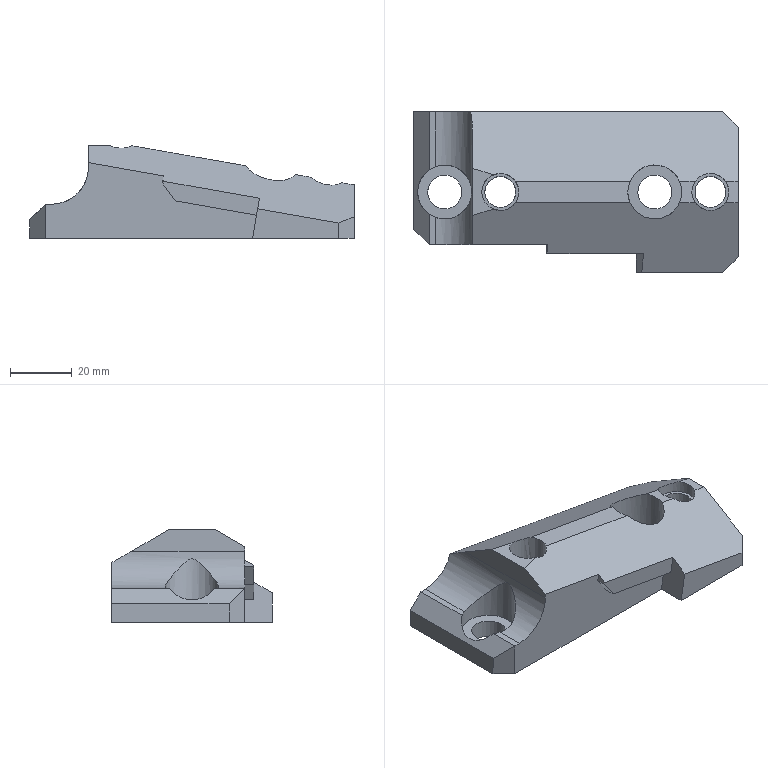Part | NX | features solid 2 | 1 solid | 37 faces | box 105 x 52 x 30.034 mm | volume 76466 mm3 | plane 28 | cylinder 7 | spline 2 | commonest cylinder face diameters 10 x2 11 x2 17.5 x2 24 x1
STEP:
#1=CARTESIAN_POINT('',(216.,165.542,-18.966));
#2=VERTEX_POINT('',#1);
#3=CARTESIAN_POINT('',(216.,129.,-18.966));
#4=VERTEX_POINT('',#3);
#5=CARTESIAN_POINT('',(216.,172.,-18.966));
#6=DIRECTION('',(0.,-1.,0.));
#7=VECTOR('',#6,1000.);
#8=LINE('',#5,#7);
#9=EDGE_CURVE('',#2,#4,#8,.T.);
#10=ORIENTED_EDGE('',*,*,#9,.F.);
#11=CARTESIAN_POINT('',(215.421,172.,-22.65));
#12=VERTEX_POINT('',#11);
#13=CARTESIAN_POINT('',(204.,169.152,-18.966));
#14=DIRECTION('',(0.1504,0.5,0.8529));
#15=DIRECTION('',(0.08682,-0.866,0.4924));
#16=AXIS2_PLACEMENT_3D('',#13,#14,#15);
#17=ELLIPSE('',#16,24.,12.);
#18=EDGE_CURVE('',#12,#2,#17,.F.);
#19=ORIENTED_EDGE('',*,*,#18,.F.);
#20=CARTESIAN_POINT('',(204.,172.,-30.966));
#21=VERTEX_POINT('',#20);
#22=CARTESIAN_POINT('',(204.,172.,-18.966));
#23=DIRECTION('',(0.,-1.,0.));
#24=DIRECTION('',(1.,0.,0.));
#25=AXIS2_PLACEMENT_3D('',#22,#23,#24);
#26=CIRCLE('',#25,12.);
#27=EDGE_CURVE('',#21,#12,#26,.T.);
#28=ORIENTED_EDGE('',*,*,#27,.F.);
#29=CARTESIAN_POINT('',(204.,154.22,-30.966));
#30=VERTEX_POINT('',#29);
#31=CARTESIAN_POINT('',(204.,172.,-30.966));
#32=DIRECTION('',(0.,-1.,0.));
#33=VECTOR('',#32,1000.);
#34=LINE('',#31,#33);
#35=EDGE_CURVE('',#21,#30,#34,.T.);
#36=ORIENTED_EDGE('',*,*,#35,.T.);
#37=CARTESIAN_POINT('',(204.,137.78,-30.966));
#38=VERTEX_POINT('',#37);
#39=CARTESIAN_POINT('',(204.,137.78,-30.966));
#40=CARTESIAN_POINT('',(205.575,137.206,-30.966));
#41=CARTESIAN_POINT('',(208.988,137.058,-30.263));
#42=CARTESIAN_POINT('',(212.178,138.742,-27.95));
#43=CARTESIAN_POINT('',(213.938,140.565,-25.79));
#44=CARTESIAN_POINT('',(214.896,142.091,-24.109));
#45=CARTESIAN_POINT('',(215.432,143.518,-22.69));
#46=CARTESIAN_POINT('',(215.694,144.818,-21.684));
#47=CARTESIAN_POINT('',(215.781,146.05,-21.25));
#48=CARTESIAN_POINT('',(215.682,147.258,-21.737));
#49=CARTESIAN_POINT('',(215.413,148.543,-22.746));
#50=CARTESIAN_POINT('',(214.875,149.952,-24.156));
#51=CARTESIAN_POINT('',(213.901,151.482,-25.843));
#52=CARTESIAN_POINT('',(212.158,153.267,-27.963));
#53=CARTESIAN_POINT('',(208.962,154.947,-30.274));
#54=CARTESIAN_POINT('',(205.569,154.792,-30.966));
#55=CARTESIAN_POINT('',(204.,154.22,-30.966));
#56=B_SPLINE_CURVE_WITH_KNOTS('',3,(#39,#40,#41,#42,#43,#44,#45,#46,#47,#48,#49,#50,#51,#52,#53,#54,#55),.UNSPECIFIED.,.F.,.F.,(4,1,1,1,1,1,1,1,1,1,1,1,1,1,4),(0.,0.004955,0.009911,0.01239,0.01487,0.01734,0.01858,0.01982,0.02106,0.0223,0.02478,0.02725,0.02973,0.03469,0.03964),.UNSPECIFIED.);
#57=EDGE_CURVE('',#38,#30,#56,.T.);
#58=ORIENTED_EDGE('',*,*,#57,.F.);
#59=CARTESIAN_POINT('',(204.,129.,-30.966));
#60=VERTEX_POINT('',#59);
#61=CARTESIAN_POINT('',(204.,172.,-30.966));
#62=DIRECTION('',(0.,-1.,0.));
#63=VECTOR('',#62,1000.);
#64=LINE('',#61,#63);
#65=EDGE_CURVE('',#38,#60,#64,.T.);
#66=ORIENTED_EDGE('',*,*,#65,.T.);
#67=CARTESIAN_POINT('',(204.,129.,-18.966));
#68=DIRECTION('',(0.,-1.,0.));
#69=DIRECTION('',(0.,0.,-1.));
#70=AXIS2_PLACEMENT_3D('',#67,#68,#69);
#71=CIRCLE('',#70,12.);
#72=EDGE_CURVE('',#60,#4,#71,.T.);
#73=ORIENTED_EDGE('',*,*,#72,.T.);
#74=EDGE_LOOP('',(#10,#19,#28,#36,#58,#66,#73));
#75=FACE_BOUND('',#74,.T.);
#76=CARTESIAN_POINT('',(204.,172.,-18.966));
#77=DIRECTION('',(0.,-1.,0.));
#78=DIRECTION('',(0.,0.,1.));
#79=AXIS2_PLACEMENT_3D('',#76,#77,#78);
#80=CYLINDRICAL_SURFACE('',#79,12.);
#81=ADVANCED_FACE('',(#75),#80,.F.);
#82=CARTESIAN_POINT('',(244.012,129.,-29.844));
#83=VERTEX_POINT('',#82);
#84=CARTESIAN_POINT('',(270.401,129.,-34.497));
#85=VERTEX_POINT('',#84);
#86=CARTESIAN_POINT('',(194.772,129.,-21.162));
#87=DIRECTION('',(0.9848,0.,-0.1736));
#88=VECTOR('',#87,1000.);
#89=LINE('',#86,#88);
#90=EDGE_CURVE('',#83,#85,#89,.T.);
#91=ORIENTED_EDGE('',*,*,#90,.T.);
#92=CARTESIAN_POINT('',(270.401,126.,-34.497));
#93=VERTEX_POINT('',#92);
#94=CARTESIAN_POINT('',(270.401,120.,-34.497));
#95=DIRECTION('',(0.,1.,0.));
#96=VECTOR('',#95,1000.);
#97=LINE('',#94,#96);
#98=EDGE_CURVE('',#93,#85,#97,.T.);
#99=ORIENTED_EDGE('',*,*,#98,.F.);
#100=CARTESIAN_POINT('',(244.012,126.,-29.844));
#101=VERTEX_POINT('',#100);
#102=CARTESIAN_POINT('',(194.772,126.,-21.162));
#103=DIRECTION('',(0.9848,0.,-0.1736));
#104=VECTOR('',#103,1000.);
#105=LINE('',#102,#104);
#106=EDGE_CURVE('',#101,#93,#105,.T.);
#107=ORIENTED_EDGE('',*,*,#106,.F.);
#108=CARTESIAN_POINT('',(244.012,126.,-29.844));
#109=DIRECTION('',(0.,-1.,0.));
#110=VECTOR('',#109,1000.);
#111=LINE('',#108,#110);
#112=EDGE_CURVE('',#83,#101,#111,.T.);
#113=ORIENTED_EDGE('',*,*,#112,.F.);
#114=EDGE_LOOP('',(#91,#99,#107,#113));
#115=FACE_BOUND('',#114,.T.);
#116=CARTESIAN_POINT('',(194.772,120.,-21.162));
#117=DIRECTION('',(-0.1736,0.,-0.9848));
#118=DIRECTION('',(-0.9848,0.,0.1736));
#119=AXIS2_PLACEMENT_3D('',#116,#117,#118);
#120=PLANE('',#119);
#121=ADVANCED_FACE('',(#115),#120,.T.);
#122=CARTESIAN_POINT('',(269.078,120.,-42.));
#123=VERTEX_POINT('',#122);
#124=CARTESIAN_POINT('',(297.,120.,-42.));
#125=VERTEX_POINT('',#124);
#126=CARTESIAN_POINT('',(166.772,120.,-42.));
#127=DIRECTION('',(1.,0.,0.));
#128=VECTOR('',#127,1000.);
#129=LINE('',#126,#128);
#130=EDGE_CURVE('',#123,#125,#129,.T.);
#131=ORIENTED_EDGE('',*,*,#130,.T.);
#132=CARTESIAN_POINT('',(297.,120.,-37.034));
#133=VERTEX_POINT('',#132);
#134=CARTESIAN_POINT('',(297.,120.,-42.966));
#135=DIRECTION('',(0.,0.,-1.));
#136=VECTOR('',#135,1000.);
#137=LINE('',#134,#136);
#138=EDGE_CURVE('',#133,#125,#137,.T.);
#139=ORIENTED_EDGE('',*,*,#138,.F.);
#140=CARTESIAN_POINT('',(270.769,120.,-32.409));
#141=VERTEX_POINT('',#140);
#142=CARTESIAN_POINT('',(172.845,120.,-15.142));
#143=DIRECTION('',(0.9848,0.,-0.1736));
#144=VECTOR('',#143,1000.);
#145=LINE('',#142,#144);
#146=EDGE_CURVE('',#141,#133,#145,.T.);
#147=ORIENTED_EDGE('',*,*,#146,.F.);
#148=CARTESIAN_POINT('',(259.982,120.,-93.586));
#149=DIRECTION('',(0.1736,0.,0.9848));
#150=VECTOR('',#149,1000.);
#151=LINE('',#148,#150);
#152=EDGE_CURVE('',#123,#141,#151,.T.);
#153=ORIENTED_EDGE('',*,*,#152,.F.);
#154=EDGE_LOOP('',(#131,#139,#147,#153));
#155=FACE_BOUND('',#154,.T.);
#156=CARTESIAN_POINT('',(166.772,120.,-49.585));
#157=DIRECTION('',(0.,-1.,0.));
#158=DIRECTION('',(0.,0.,1.));
#159=AXIS2_PLACEMENT_3D('',#156,#157,#158);
#160=PLANE('',#159);
#161=ADVANCED_FACE('',(#155),#160,.T.);
#162=CARTESIAN_POINT('',(302.,142.536,-24.704));
#163=VERTEX_POINT('',#162);
#164=CARTESIAN_POINT('',(302.,125.,-34.985));
#165=VERTEX_POINT('',#164);
#166=CARTESIAN_POINT('',(302.,130.815,-31.576));
#167=DIRECTION('',(0.,-0.8627,-0.5058));
#168=VECTOR('',#167,1000.);
#169=LINE('',#166,#168);
#170=EDGE_CURVE('',#163,#165,#169,.T.);
#171=ORIENTED_EDGE('',*,*,#170,.F.);
#172=CARTESIAN_POINT('',(297.897,142.536,-23.981));
#173=VERTEX_POINT('',#172);
#174=CARTESIAN_POINT('',(175.104,142.536,-2.329));
#175=DIRECTION('',(0.9848,0.,-0.1736));
#176=VECTOR('',#175,1000.);
#177=LINE('',#174,#176);
#178=EDGE_CURVE('',#173,#163,#177,.T.);
#179=ORIENTED_EDGE('',*,*,#178,.F.);
#180=CARTESIAN_POINT('',(288.103,142.536,-22.254));
#181=VERTEX_POINT('',#180);
#182=CARTESIAN_POINT('',(297.897,142.536,-23.981));
#183=CARTESIAN_POINT('',(297.358,141.77,-24.335));
#184=CARTESIAN_POINT('',(295.85,140.432,-24.853));
#185=CARTESIAN_POINT('',(292.773,139.747,-24.712));
#186=CARTESIAN_POINT('',(289.937,140.598,-23.713));
#187=CARTESIAN_POINT('',(288.601,141.828,-22.757));
#188=CARTESIAN_POINT('',(288.103,142.536,-22.254));
#189=B_SPLINE_CURVE_WITH_KNOTS('',3,(#182,#183,#184,#185,#186,#187,#188),.UNSPECIFIED.,.F.,.F.,(4,1,1,1,4),(0.006466,0.009441,0.01242,0.01539,0.01837),.UNSPECIFIED.);
#190=EDGE_CURVE('',#173,#181,#189,.T.);
#191=ORIENTED_EDGE('',*,*,#190,.T.);
#192=CARTESIAN_POINT('',(283.035,142.536,-21.36));
#193=VERTEX_POINT('',#192);
#194=CARTESIAN_POINT('',(175.104,142.536,-2.329));
#195=DIRECTION('',(0.9848,0.,-0.1736));
#196=VECTOR('',#195,1000.);
#197=LINE('',#194,#196);
#198=EDGE_CURVE('',#193,#181,#197,.T.);
#199=ORIENTED_EDGE('',*,*,#198,.F.);
#200=CARTESIAN_POINT('',(266.965,142.536,-18.527));
#201=VERTEX_POINT('',#200);
#202=CARTESIAN_POINT('',(275.,146.,-17.912));
#203=DIRECTION('',(0.1504,-0.5,0.8529));
#204=DIRECTION('',(0.2456,-0.8167,-0.5221));
#205=AXIS2_PLACEMENT_3D('',#202,#203,#204);
#206=ELLIPSE('',#205,10.259,8.75);
#207=EDGE_CURVE('',#193,#201,#206,.F.);
#208=ORIENTED_EDGE('',*,*,#207,.T.);
#209=CARTESIAN_POINT('',(229.897,142.536,-11.99));
#210=VERTEX_POINT('',#209);
#211=CARTESIAN_POINT('',(175.104,142.536,-2.329));
#212=DIRECTION('',(0.9848,0.,-0.1736));
#213=VECTOR('',#212,1000.);
#214=LINE('',#211,#213);
#215=EDGE_CURVE('',#210,#201,#214,.T.);
#216=ORIENTED_EDGE('',*,*,#215,.F.);
#217=CARTESIAN_POINT('',(222.769,140.434,-11.966));
#218=VERTEX_POINT('',#217);
#219=CARTESIAN_POINT('',(229.897,142.536,-11.99));
#220=CARTESIAN_POINT('',(229.158,141.486,-12.476));
#221=CARTESIAN_POINT('',(226.837,139.774,-13.07));
#222=CARTESIAN_POINT('',(223.955,139.958,-12.454));
#223=CARTESIAN_POINT('',(222.769,140.434,-11.966));
#224=B_SPLINE_CURVE_WITH_KNOTS('',3,(#219,#220,#221,#222,#223),.UNSPECIFIED.,.F.,.F.,(4,1,4),(0.0002423,0.004332,0.008422),.UNSPECIFIED.);
#225=EDGE_CURVE('',#210,#218,#224,.T.);
#226=ORIENTED_EDGE('',*,*,#225,.T.);
#227=CARTESIAN_POINT('',(216.,138.398,-11.966));
#228=VERTEX_POINT('',#227);
#229=CARTESIAN_POINT('',(171.676,125.067,-11.966));
#230=DIRECTION('',(-0.9576,-0.288,0.));
#231=VECTOR('',#230,1000.);
#232=LINE('',#229,#231);
#233=EDGE_CURVE('',#218,#228,#232,.T.);
#234=ORIENTED_EDGE('',*,*,#233,.T.);
#235=CARTESIAN_POINT('',(216.,129.,-17.476));
#236=VERTEX_POINT('',#235);
#237=CARTESIAN_POINT('',(216.,124.198,-20.29));
#238=DIRECTION('',(0.,-0.8627,-0.5058));
#239=VECTOR('',#238,1000.);
#240=LINE('',#237,#239);
#241=EDGE_CURVE('',#228,#236,#240,.T.);
#242=ORIENTED_EDGE('',*,*,#241,.T.);
#243=CARTESIAN_POINT('',(240.359,129.,-21.771));
#244=VERTEX_POINT('',#243);
#245=CARTESIAN_POINT('',(173.747,129.,-10.025));
#246=DIRECTION('',(-0.9848,0.,0.1736));
#247=VECTOR('',#246,1000.);
#248=LINE('',#245,#247);
#249=EDGE_CURVE('',#244,#236,#248,.T.);
#250=ORIENTED_EDGE('',*,*,#249,.F.);
#251=CARTESIAN_POINT('',(240.058,126.,-23.476));
#252=VERTEX_POINT('',#251);
#253=CARTESIAN_POINT('',(239.545,120.885,-26.385));
#254=DIRECTION('',(0.08682,0.866,0.4924));
#255=VECTOR('',#254,1000.);
#256=LINE('',#253,#255);
#257=EDGE_CURVE('',#252,#244,#256,.T.);
#258=ORIENTED_EDGE('',*,*,#257,.F.);
#259=CARTESIAN_POINT('',(271.37,126.,-28.998));
#260=VERTEX_POINT('',#259);
#261=CARTESIAN_POINT('',(173.446,126.,-11.731));
#262=DIRECTION('',(0.9848,0.,-0.1736));
#263=VECTOR('',#262,1000.);
#264=LINE('',#261,#263);
#265=EDGE_CURVE('',#252,#260,#264,.T.);
#266=ORIENTED_EDGE('',*,*,#265,.T.);
#267=CARTESIAN_POINT('',(270.857,120.885,-31.906));
#268=DIRECTION('',(0.08682,0.866,0.4924));
#269=VECTOR('',#268,1000.);
#270=LINE('',#267,#269);
#271=EDGE_CURVE('',#141,#260,#270,.T.);
#272=ORIENTED_EDGE('',*,*,#271,.F.);
#273=ORIENTED_EDGE('',*,*,#146,.T.);
#274=CARTESIAN_POINT('',(300.491,123.491,-35.603));
#275=DIRECTION('',(-0.6792,-0.6792,-0.2784));
#276=VECTOR('',#275,1000.);
#277=LINE('',#274,#276);
#278=EDGE_CURVE('',#165,#133,#277,.T.);
#279=ORIENTED_EDGE('',*,*,#278,.F.);
#280=EDGE_LOOP('',(#171,#179,#191,#199,#208,#216,#226,#234,#242,#250,#258,#266,#272,#273,#279));
#281=FACE_BOUND('',#280,.T.);
#282=CARTESIAN_POINT('',(172.934,120.885,-14.639));
#283=DIRECTION('',(-0.1504,0.5,-0.8529));
#284=DIRECTION('',(0.,-0.8627,-0.5058));
#285=AXIS2_PLACEMENT_3D('',#282,#283,#284);
#286=PLANE('',#285);
#287=ADVANCED_FACE('',(#281),#286,.F.);
#288=CARTESIAN_POINT('',(297.,172.,-37.034));
#289=VERTEX_POINT('',#288);
#290=CARTESIAN_POINT('',(172.845,172.,-15.142));
#291=DIRECTION('',(0.9848,0.,-0.1736));
#292=VECTOR('',#291,1000.);
#293=LINE('',#290,#292);
#294=EDGE_CURVE('',#12,#289,#293,.T.);
#295=ORIENTED_EDGE('',*,*,#294,.F.);
#296=ORIENTED_EDGE('',*,*,#18,.T.);
#297=CARTESIAN_POINT('',(216.,153.602,-11.966));
#298=VERTEX_POINT('',#297);
#299=CARTESIAN_POINT('',(216.,167.802,-20.29));
#300=DIRECTION('',(0.,-0.8627,0.5058));
#301=VECTOR('',#300,1000.);
#302=LINE('',#299,#301);
#303=EDGE_CURVE('',#2,#298,#302,.T.);
#304=ORIENTED_EDGE('',*,*,#303,.T.);
#305=CARTESIAN_POINT('',(222.769,151.566,-11.966));
#306=VERTEX_POINT('',#305);
#307=CARTESIAN_POINT('',(171.676,166.933,-11.966));
#308=DIRECTION('',(0.9576,-0.288,0.));
#309=VECTOR('',#308,1000.);
#310=LINE('',#307,#309);
#311=EDGE_CURVE('',#298,#306,#310,.T.);
#312=ORIENTED_EDGE('',*,*,#311,.T.);
#313=CARTESIAN_POINT('',(229.897,149.464,-11.99));
#314=VERTEX_POINT('',#313);
#315=CARTESIAN_POINT('',(222.769,151.566,-11.966));
#316=CARTESIAN_POINT('',(223.949,152.039,-12.451));
#317=CARTESIAN_POINT('',(226.819,152.232,-13.07));
#318=CARTESIAN_POINT('',(229.155,150.519,-12.478));
#319=CARTESIAN_POINT('',(229.897,149.464,-11.99));
#320=B_SPLINE_CURVE_WITH_KNOTS('',3,(#315,#316,#317,#318,#319),.UNSPECIFIED.,.F.,.F.,(4,1,4),(0.003035,0.007118,0.0112),.UNSPECIFIED.);
#321=EDGE_CURVE('',#306,#314,#320,.T.);
#322=ORIENTED_EDGE('',*,*,#321,.T.);
#323=CARTESIAN_POINT('',(266.965,149.464,-18.527));
#324=VERTEX_POINT('',#323);
#325=CARTESIAN_POINT('',(175.104,149.464,-2.329));
#326=DIRECTION('',(0.9848,0.,-0.1736));
#327=VECTOR('',#326,1000.);
#328=LINE('',#325,#327);
#329=EDGE_CURVE('',#314,#324,#328,.T.);
#330=ORIENTED_EDGE('',*,*,#329,.T.);
#331=CARTESIAN_POINT('',(283.035,149.464,-21.36));
#332=VERTEX_POINT('',#331);
#333=CARTESIAN_POINT('',(275.,146.,-17.912));
#334=DIRECTION('',(0.1504,0.5,0.8529));
#335=DIRECTION('',(0.2456,0.8167,-0.5221));
#336=AXIS2_PLACEMENT_3D('',#333,#334,#335);
#337=ELLIPSE('',#336,10.259,8.75);
#338=EDGE_CURVE('',#324,#332,#337,.F.);
#339=ORIENTED_EDGE('',*,*,#338,.T.);
#340=CARTESIAN_POINT('',(288.103,149.464,-22.254));
#341=VERTEX_POINT('',#340);
#342=CARTESIAN_POINT('',(175.104,149.464,-2.329));
#343=DIRECTION('',(0.9848,0.,-0.1736));
#344=VECTOR('',#343,1000.);
#345=LINE('',#342,#344);
#346=EDGE_CURVE('',#332,#341,#345,.T.);
#347=ORIENTED_EDGE('',*,*,#346,.T.);
#348=CARTESIAN_POINT('',(297.897,149.464,-23.981));
#349=VERTEX_POINT('',#348);
#350=CARTESIAN_POINT('',(288.103,149.464,-22.254));
#351=CARTESIAN_POINT('',(288.605,150.178,-22.761));
#352=CARTESIAN_POINT('',(289.93,151.394,-23.707));
#353=CARTESIAN_POINT('',(292.755,152.25,-24.707));
#354=CARTESIAN_POINT('',(295.825,151.583,-24.858));
#355=CARTESIAN_POINT('',(297.355,150.233,-24.336));
#356=CARTESIAN_POINT('',(297.897,149.464,-23.981));
#357=B_SPLINE_CURVE_WITH_KNOTS('',3,(#350,#351,#352,#353,#354,#355,#356),.UNSPECIFIED.,.F.,.F.,(4,1,1,1,4),(0.005558,0.008538,0.01152,0.0145,0.01748),.UNSPECIFIED.);
#358=EDGE_CURVE('',#341,#349,#357,.T.);
#359=ORIENTED_EDGE('',*,*,#358,.T.);
#360=CARTESIAN_POINT('',(302.,149.464,-24.704));
#361=VERTEX_POINT('',#360);
#362=CARTESIAN_POINT('',(175.104,149.464,-2.329));
#363=DIRECTION('',(0.9848,0.,-0.1736));
#364=VECTOR('',#363,1000.);
#365=LINE('',#362,#364);
#366=EDGE_CURVE('',#349,#361,#365,.T.);
#367=ORIENTED_EDGE('',*,*,#366,.T.);
#368=CARTESIAN_POINT('',(302.,167.,-34.985));
#369=VERTEX_POINT('',#368);
#370=CARTESIAN_POINT('',(302.,161.185,-31.576));
#371=DIRECTION('',(0.,-0.8627,0.5058));
#372=VECTOR('',#371,1000.);
#373=LINE('',#370,#372);
#374=EDGE_CURVE('',#369,#361,#373,.T.);
#375=ORIENTED_EDGE('',*,*,#374,.F.);
#376=CARTESIAN_POINT('',(300.491,168.509,-35.603));
#377=DIRECTION('',(0.6792,-0.6792,0.2784));
#378=VECTOR('',#377,1000.);
#379=LINE('',#376,#378);
#380=EDGE_CURVE('',#289,#369,#379,.T.);
#381=ORIENTED_EDGE('',*,*,#380,.F.);
#382=EDGE_LOOP('',(#295,#296,#304,#312,#322,#330,#339,#347,#359,#367,#375,#381));
#383=FACE_BOUND('',#382,.T.);
#384=CARTESIAN_POINT('',(172.934,171.115,-14.639));
#385=DIRECTION('',(-0.1504,-0.5,-0.8529));
#386=DIRECTION('',(0.,-0.8627,0.5058));
#387=AXIS2_PLACEMENT_3D('',#384,#385,#386);
#388=PLANE('',#387);
#389=ADVANCED_FACE('',(#383),#388,.F.);
#390=CARTESIAN_POINT('',(229.897,149.464,-11.99));
#391=CARTESIAN_POINT('',(230.61,148.453,-12.116));
#392=CARTESIAN_POINT('',(231.39,146.012,-12.254));
#393=CARTESIAN_POINT('',(230.61,143.548,-12.116));
#394=CARTESIAN_POINT('',(229.897,142.536,-11.99));
#395=B_SPLINE_CURVE_WITH_KNOTS('',3,(#390,#391,#392,#393,#394),.UNSPECIFIED.,.F.,.F.,(4,1,4),(0.,0.003679,0.007357),.UNSPECIFIED.);
#396=EDGE_CURVE('',#314,#210,#395,.T.);
#397=ORIENTED_EDGE('',*,*,#396,.T.);
#398=ORIENTED_EDGE('',*,*,#215,.T.);
#399=CARTESIAN_POINT('',(275.,146.,-19.943));
#400=DIRECTION('',(0.1736,0.,0.9848));
#401=DIRECTION('',(0.9848,0.,-0.1736));
#402=AXIS2_PLACEMENT_3D('',#399,#400,#401);
#403=ELLIPSE('',#402,8.885,8.75);
#404=EDGE_CURVE('',#201,#324,#403,.F.);
#405=ORIENTED_EDGE('',*,*,#404,.T.);
#406=ORIENTED_EDGE('',*,*,#329,.F.);
#407=EDGE_LOOP('',(#397,#398,#405,#406));
#408=FACE_BOUND('',#407,.T.);
#409=CARTESIAN_POINT('',(175.104,149.464,-2.329));
#410=DIRECTION('',(-0.1736,0.,-0.9848));
#411=DIRECTION('',(-0.9848,0.,0.1736));
#412=AXIS2_PLACEMENT_3D('',#409,#410,#411);
#413=PLANE('',#412);
#414=ADVANCED_FACE('',(#408),#413,.F.);
#415=ORIENTED_EDGE('',*,*,#311,.F.);
#416=CARTESIAN_POINT('',(216.,172.,-11.966));
#417=DIRECTION('',(0.,-1.,0.));
#418=VECTOR('',#417,1000.);
#419=LINE('',#416,#418);
#420=EDGE_CURVE('',#298,#228,#419,.T.);
#421=ORIENTED_EDGE('',*,*,#420,.T.);
#422=ORIENTED_EDGE('',*,*,#233,.F.);
#423=CARTESIAN_POINT('',(231.,147.58,-11.966));
#424=CARTESIAN_POINT('',(231.,144.42,-11.966));
#425=CARTESIAN_POINT('',(230.36,142.875,-11.966));
#426=CARTESIAN_POINT('',(228.125,140.64,-11.966));
#427=CARTESIAN_POINT('',(226.58,140.,-11.966));
#428=CARTESIAN_POINT('',(223.42,140.,-11.966));
#429=CARTESIAN_POINT('',(221.875,140.64,-11.966));
#430=CARTESIAN_POINT('',(219.64,142.875,-11.966));
#431=CARTESIAN_POINT('',(219.,144.42,-11.966));
#432=CARTESIAN_POINT('',(219.,147.58,-11.966));
#433=CARTESIAN_POINT('',(219.64,149.125,-11.966));
#434=CARTESIAN_POINT('',(221.875,151.36,-11.966));
#435=CARTESIAN_POINT('',(223.42,152.,-11.966));
#436=CARTESIAN_POINT('',(226.58,152.,-11.966));
#437=CARTESIAN_POINT('',(228.125,151.36,-11.966));
#438=CARTESIAN_POINT('',(230.36,149.125,-11.966));
#439=CARTESIAN_POINT('',(231.,147.58,-11.966));
#440=CARTESIAN_POINT('',(231.,144.42,-11.966));
#441=B_SPLINE_CURVE_WITH_KNOTS('',3,(#423,#424,#425,#426,#427,#428,#429,#430,#431,#432,#433,#434,#435,#436,#437,#438,#439,#440),.UNSPECIFIED.,.T.,.F.,(2,2,2,2,2,2,2,2,2,2,2),(-0.125,0.,0.125,0.25,0.375,0.5,0.625,0.75,0.875,1.,1.125),.UNSPECIFIED.);
#442=EDGE_CURVE('',#306,#218,#441,.F.);
#443=ORIENTED_EDGE('',*,*,#442,.F.);
#444=EDGE_LOOP('',(#415,#421,#422,#443));
#445=FACE_BOUND('',#444,.T.);
#446=CARTESIAN_POINT('',(216.,172.,-11.966));
#447=DIRECTION('',(0.,0.,1.));
#448=DIRECTION('',(0.,1.,0.));
#449=AXIS2_PLACEMENT_3D('',#446,#447,#448);
#450=PLANE('',#449);
#451=ADVANCED_FACE('',(#445),#450,.T.);
#452=CARTESIAN_POINT('',(288.103,142.536,-22.254));
#453=CARTESIAN_POINT('',(287.39,143.547,-22.128));
#454=CARTESIAN_POINT('',(286.61,145.988,-21.99));
#455=CARTESIAN_POINT('',(287.39,148.452,-22.128));
#456=CARTESIAN_POINT('',(288.103,149.464,-22.254));
#457=B_SPLINE_CURVE_WITH_KNOTS('',3,(#452,#453,#454,#455,#456),.UNSPECIFIED.,.F.,.F.,(4,1,4),(0.,0.003679,0.007357),.UNSPECIFIED.);
#458=EDGE_CURVE('',#181,#341,#457,.T.);
#459=ORIENTED_EDGE('',*,*,#458,.T.);
#460=ORIENTED_EDGE('',*,*,#346,.F.);
#461=CARTESIAN_POINT('',(275.,146.,-19.943));
#462=DIRECTION('',(0.1736,0.,0.9848));
#463=DIRECTION('',(0.9848,0.,-0.1736));
#464=AXIS2_PLACEMENT_3D('',#461,#462,#463);
#465=ELLIPSE('',#464,8.885,8.75);
#466=EDGE_CURVE('',#332,#193,#465,.F.);
#467=ORIENTED_EDGE('',*,*,#466,.T.);
#468=ORIENTED_EDGE('',*,*,#198,.T.);
#469=EDGE_LOOP('',(#459,#460,#467,#468));
#470=FACE_BOUND('',#469,.T.);
#471=CARTESIAN_POINT('',(175.104,149.464,-2.329));
#472=DIRECTION('',(-0.1736,0.,-0.9848));
#473=DIRECTION('',(-0.9848,0.,0.1736));
#474=AXIS2_PLACEMENT_3D('',#471,#472,#473);
#475=PLANE('',#474);
#476=ADVANCED_FACE('',(#470),#475,.F.);
#477=CARTESIAN_POINT('',(297.897,149.464,-23.981));
#478=CARTESIAN_POINT('',(298.61,148.453,-24.106));
#479=CARTESIAN_POINT('',(299.39,146.012,-24.244));
#480=CARTESIAN_POINT('',(298.61,143.548,-24.106));
#481=CARTESIAN_POINT('',(297.897,142.536,-23.981));
#482=B_SPLINE_CURVE_WITH_KNOTS('',3,(#477,#478,#479,#480,#481),.UNSPECIFIED.,.F.,.F.,(4,1,4),(0.,0.003679,0.007357),.UNSPECIFIED.);
#483=EDGE_CURVE('',#349,#173,#482,.T.);
#484=ORIENTED_EDGE('',*,*,#483,.T.);
#485=ORIENTED_EDGE('',*,*,#178,.T.);
#486=CARTESIAN_POINT('',(302.,149.464,-24.704));
#487=DIRECTION('',(0.,-1.,0.));
#488=VECTOR('',#487,1000.);
#489=LINE('',#486,#488);
#490=EDGE_CURVE('',#361,#163,#489,.T.);
#491=ORIENTED_EDGE('',*,*,#490,.F.);
#492=ORIENTED_EDGE('',*,*,#366,.F.);
#493=EDGE_LOOP('',(#484,#485,#491,#492));
#494=FACE_BOUND('',#493,.T.);
#495=CARTESIAN_POINT('',(175.104,149.464,-2.329));
#496=DIRECTION('',(-0.1736,0.,-0.9848));
#497=DIRECTION('',(-0.9848,0.,0.1736));
#498=AXIS2_PLACEMENT_3D('',#495,#496,#497);
#499=PLANE('',#498);
#500=ADVANCED_FACE('',(#494),#499,.F.);
#501=CARTESIAN_POINT('',(215.75,146.,-35.966));
#502=VERTEX_POINT('',#501);
#503=CARTESIAN_POINT('',(207.,146.,-35.966));
#504=DIRECTION('',(0.,0.,-1.));
#505=DIRECTION('',(1.,0.,0.));
#506=AXIS2_PLACEMENT_3D('',#503,#504,#505);
#507=CIRCLE('',#506,8.75);
#508=EDGE_CURVE('',#502,#502,#507,.T.);
#509=ORIENTED_EDGE('',*,*,#508,.F.);
#510=EDGE_LOOP('',(#509));
#511=FACE_BOUND('',#510,.T.);
#512=CARTESIAN_POINT('',(212.5,146.,-35.966));
#513=VERTEX_POINT('',#512);
#514=CARTESIAN_POINT('',(207.,146.,-35.966));
#515=DIRECTION('',(0.,0.,-1.));
#516=DIRECTION('',(1.,0.,0.));
#517=AXIS2_PLACEMENT_3D('',#514,#515,#516);
#518=CIRCLE('',#517,5.5);
#519=EDGE_CURVE('',#513,#513,#518,.F.);
#520=ORIENTED_EDGE('',*,*,#519,.F.);
#521=EDGE_LOOP('',(#520));
#522=FACE_BOUND('',#521,.T.);
#523=CARTESIAN_POINT('',(207.,146.,-35.966));
#524=DIRECTION('',(0.,0.,1.));
#525=DIRECTION('',(1.,0.,0.));
#526=AXIS2_PLACEMENT_3D('',#523,#524,#525);
#527=PLANE('',#526);
#528=ADVANCED_FACE('',(#511,#522),#527,.T.);
#529=CARTESIAN_POINT('',(283.75,146.,-35.966));
#530=VERTEX_POINT('',#529);
#531=CARTESIAN_POINT('',(275.,146.,-35.966));
#532=DIRECTION('',(0.,0.,-1.));
#533=DIRECTION('',(1.,0.,0.));
#534=AXIS2_PLACEMENT_3D('',#531,#532,#533);
#535=CIRCLE('',#534,8.75);
#536=EDGE_CURVE('',#530,#530,#535,.T.);
#537=ORIENTED_EDGE('',*,*,#536,.F.);
#538=EDGE_LOOP('',(#537));
#539=FACE_BOUND('',#538,.T.);
#540=CARTESIAN_POINT('',(280.5,146.,-35.966));
#541=VERTEX_POINT('',#540);
#542=CARTESIAN_POINT('',(275.,146.,-35.966));
#543=DIRECTION('',(0.,0.,-1.));
#544=DIRECTION('',(1.,0.,0.));
#545=AXIS2_PLACEMENT_3D('',#542,#543,#544);
#546=CIRCLE('',#545,5.5);
#547=EDGE_CURVE('',#541,#541,#546,.F.);
#548=ORIENTED_EDGE('',*,*,#547,.F.);
#549=EDGE_LOOP('',(#548));
#550=FACE_BOUND('',#549,.T.);
#551=CARTESIAN_POINT('',(275.,146.,-35.966));
#552=DIRECTION('',(0.,0.,1.));
#553=DIRECTION('',(1.,0.,0.));
#554=AXIS2_PLACEMENT_3D('',#551,#552,#553);
#555=PLANE('',#554);
#556=ADVANCED_FACE('',(#539,#550),#555,.T.);
#557=CARTESIAN_POINT('',(202.,138.819,-30.966));
#558=VERTEX_POINT('',#557);
#559=CARTESIAN_POINT('',(202.,129.,-30.966));
#560=VERTEX_POINT('',#559);
#561=CARTESIAN_POINT('',(202.,172.,-30.966));
#562=DIRECTION('',(0.,-1.,0.));
#563=VECTOR('',#562,1000.);
#564=LINE('',#561,#563);
#565=EDGE_CURVE('',#558,#560,#564,.T.);
#566=ORIENTED_EDGE('',*,*,#565,.F.);
#567=CARTESIAN_POINT('',(202.,153.181,-30.966));
#568=VERTEX_POINT('',#567);
#569=CARTESIAN_POINT('',(207.,146.,-25.966));
#570=DIRECTION('',(0.7071,0.,-0.7071));
#571=DIRECTION('',(-0.7071,0.,-0.7071));
#572=AXIS2_PLACEMENT_3D('',#569,#570,#571);
#573=ELLIPSE('',#572,12.374,8.75);
#574=EDGE_CURVE('',#568,#558,#573,.F.);
#575=ORIENTED_EDGE('',*,*,#574,.F.);
#576=CARTESIAN_POINT('',(202.,172.,-30.966));
#577=VERTEX_POINT('',#576);
#578=CARTESIAN_POINT('',(202.,172.,-30.966));
#579=DIRECTION('',(0.,-1.,0.));
#580=VECTOR('',#579,1000.);
#581=LINE('',#578,#580);
#582=EDGE_CURVE('',#577,#568,#581,.T.);
#583=ORIENTED_EDGE('',*,*,#582,.F.);
#584=CARTESIAN_POINT('',(197.,172.,-35.966));
#585=VERTEX_POINT('',#584);
#586=CARTESIAN_POINT('',(197.,172.,-35.966));
#587=DIRECTION('',(0.7071,0.,0.7071));
#588=VECTOR('',#587,1000.);
#589=LINE('',#586,#588);
#590=EDGE_CURVE('',#585,#577,#589,.T.);
#591=ORIENTED_EDGE('',*,*,#590,.F.);
#592=CARTESIAN_POINT('',(197.,134.,-35.966));
#593=VERTEX_POINT('',#592);
#594=CARTESIAN_POINT('',(197.,172.,-35.966));
#595=DIRECTION('',(0.,-1.,0.));
#596=VECTOR('',#595,1000.);
#597=LINE('',#594,#596);
#598=EDGE_CURVE('',#585,#593,#597,.T.);
#599=ORIENTED_EDGE('',*,*,#598,.T.);
#600=CARTESIAN_POINT('',(184.333,146.667,-48.633));
#601=DIRECTION('',(0.5774,-0.5774,0.5774));
#602=VECTOR('',#601,1000.);
#603=LINE('',#600,#602);
#604=EDGE_CURVE('',#560,#593,#603,.F.);
#605=ORIENTED_EDGE('',*,*,#604,.F.);
#606=EDGE_LOOP('',(#566,#575,#583,#591,#599,#605));
#607=FACE_BOUND('',#606,.T.);
#608=CARTESIAN_POINT('',(197.,172.,-35.966));
#609=DIRECTION('',(-0.7071,0.,0.7071));
#610=DIRECTION('',(0.7071,0.,0.7071));
#611=AXIS2_PLACEMENT_3D('',#608,#609,#610);
#612=PLANE('',#611);
#613=ADVANCED_FACE('',(#607),#612,.T.);
#614=ORIENTED_EDGE('',*,*,#35,.F.);
#615=CARTESIAN_POINT('',(202.,172.,-30.966));
#616=DIRECTION('',(1.,0.,0.));
#617=VECTOR('',#616,1000.);
#618=LINE('',#615,#617);
#619=EDGE_CURVE('',#577,#21,#618,.T.);
#620=ORIENTED_EDGE('',*,*,#619,.F.);
#621=ORIENTED_EDGE('',*,*,#582,.T.);
#622=CARTESIAN_POINT('',(207.,146.,-30.966));
#623=DIRECTION('',(0.,0.,-1.));
#624=DIRECTION('',(1.,0.,0.));
#625=AXIS2_PLACEMENT_3D('',#622,#623,#624);
#626=CIRCLE('',#625,8.75);
#627=EDGE_CURVE('',#30,#568,#626,.F.);
#628=ORIENTED_EDGE('',*,*,#627,.F.);
#629=EDGE_LOOP('',(#614,#620,#621,#628));
#630=FACE_BOUND('',#629,.T.);
#631=CARTESIAN_POINT('',(202.,172.,-30.966));
#632=DIRECTION('',(0.,0.,1.));
#633=DIRECTION('',(1.,0.,0.));
#634=AXIS2_PLACEMENT_3D('',#631,#632,#633);
#635=PLANE('',#634);
#636=ADVANCED_FACE('',(#630),#635,.T.);
#637=CARTESIAN_POINT('',(202.,129.,-30.966));
#638=DIRECTION('',(1.,0.,0.));
#639=VECTOR('',#638,1000.);
#640=LINE('',#637,#639);
#641=EDGE_CURVE('',#560,#60,#640,.T.);
#642=ORIENTED_EDGE('',*,*,#641,.T.);
#643=ORIENTED_EDGE('',*,*,#65,.F.);
#644=CARTESIAN_POINT('',(207.,146.,-30.966));
#645=DIRECTION('',(0.,0.,-1.));
#646=DIRECTION('',(1.,0.,0.));
#647=AXIS2_PLACEMENT_3D('',#644,#645,#646);
#648=CIRCLE('',#647,8.75);
#649=EDGE_CURVE('',#558,#38,#648,.F.);
#650=ORIENTED_EDGE('',*,*,#649,.F.);
#651=ORIENTED_EDGE('',*,*,#565,.T.);
#652=EDGE_LOOP('',(#642,#643,#650,#651));
#653=FACE_BOUND('',#652,.T.);
#654=CARTESIAN_POINT('',(202.,172.,-30.966));
#655=DIRECTION('',(0.,0.,1.));
#656=DIRECTION('',(1.,0.,0.));
#657=AXIS2_PLACEMENT_3D('',#654,#655,#656);
#658=PLANE('',#657);
#659=ADVANCED_FACE('',(#653),#658,.T.);
#660=CARTESIAN_POINT('',(197.,134.,-42.));
#661=VERTEX_POINT('',#660);
#662=CARTESIAN_POINT('',(197.,134.,-35.966));
#663=DIRECTION('',(0.,0.,-1.));
#664=VECTOR('',#663,1000.);
#665=LINE('',#662,#664);
#666=EDGE_CURVE('',#593,#661,#665,.T.);
#667=ORIENTED_EDGE('',*,*,#666,.F.);
#668=ORIENTED_EDGE('',*,*,#598,.F.);
#669=CARTESIAN_POINT('',(197.,172.,-42.));
#670=VERTEX_POINT('',#669);
#671=CARTESIAN_POINT('',(197.,172.,-15.142));
#672=DIRECTION('',(0.,0.,1.));
#673=VECTOR('',#672,1000.);
#674=LINE('',#671,#673);
#675=EDGE_CURVE('',#670,#585,#674,.T.);
#676=ORIENTED_EDGE('',*,*,#675,.F.);
#677=CARTESIAN_POINT('',(197.,172.,-42.));
#678=DIRECTION('',(0.,-1.,0.));
#679=VECTOR('',#678,1000.);
#680=LINE('',#677,#679);
#681=EDGE_CURVE('',#670,#661,#680,.T.);
#682=ORIENTED_EDGE('',*,*,#681,.T.);
#683=EDGE_LOOP('',(#667,#668,#676,#682));
#684=FACE_BOUND('',#683,.T.);
#685=CARTESIAN_POINT('',(197.,172.,-35.966));
#686=DIRECTION('',(1.,0.,0.));
#687=DIRECTION('',(0.,-1.,0.));
#688=AXIS2_PLACEMENT_3D('',#685,#686,#687);
#689=PLANE('',#688);
#690=ADVANCED_FACE('',(#684),#689,.F.);
#691=CARTESIAN_POINT('',(297.,172.,-42.));
#692=VERTEX_POINT('',#691);
#693=CARTESIAN_POINT('',(172.845,172.,-42.));
#694=DIRECTION('',(-1.,0.,0.));
#695=VECTOR('',#694,1000.);
#696=LINE('',#693,#695);
#697=EDGE_CURVE('',#692,#670,#696,.T.);
#698=ORIENTED_EDGE('',*,*,#697,.T.);
#699=ORIENTED_EDGE('',*,*,#675,.T.);
#700=ORIENTED_EDGE('',*,*,#590,.T.);
#701=ORIENTED_EDGE('',*,*,#619,.T.);
#702=ORIENTED_EDGE('',*,*,#27,.T.);
#703=ORIENTED_EDGE('',*,*,#294,.T.);
#704=CARTESIAN_POINT('',(297.,172.,-37.916));
#705=DIRECTION('',(0.,0.,1.));
#706=VECTOR('',#705,1000.);
#707=LINE('',#704,#706);
#708=EDGE_CURVE('',#692,#289,#707,.T.);
#709=ORIENTED_EDGE('',*,*,#708,.F.);
#710=EDGE_LOOP('',(#698,#699,#700,#701,#702,#703,#709));
#711=FACE_BOUND('',#710,.T.);
#712=CARTESIAN_POINT('',(172.845,172.,-15.142));
#713=DIRECTION('',(0.,1.,0.));
#714=DIRECTION('',(0.,0.,-1.));
#715=AXIS2_PLACEMENT_3D('',#712,#713,#714);
#716=PLANE('',#715);
#717=ADVANCED_FACE('',(#711),#716,.T.);
#718=CARTESIAN_POINT('',(302.,167.,-42.));
#719=VERTEX_POINT('',#718);
#720=CARTESIAN_POINT('',(302.,167.,-42.966));
#721=DIRECTION('',(0.,0.,-1.));
#722=VECTOR('',#721,1000.);
#723=LINE('',#720,#722);
#724=EDGE_CURVE('',#369,#719,#723,.T.);
#725=ORIENTED_EDGE('',*,*,#724,.F.);
#726=ORIENTED_EDGE('',*,*,#374,.T.);
#727=ORIENTED_EDGE('',*,*,#490,.T.);
#728=ORIENTED_EDGE('',*,*,#170,.T.);
#729=CARTESIAN_POINT('',(302.,125.,-42.));
#730=VERTEX_POINT('',#729);
#731=CARTESIAN_POINT('',(302.,125.,-37.916));
#732=DIRECTION('',(0.,0.,1.));
#733=VECTOR('',#732,1000.);
#734=LINE('',#731,#733);
#735=EDGE_CURVE('',#730,#165,#734,.T.);
#736=ORIENTED_EDGE('',*,*,#735,.F.);
#737=CARTESIAN_POINT('',(302.,172.,-42.));
#738=DIRECTION('',(0.,1.,0.));
#739=VECTOR('',#738,1000.);
#740=LINE('',#737,#739);
#741=EDGE_CURVE('',#730,#719,#740,.T.);
#742=ORIENTED_EDGE('',*,*,#741,.T.);
#743=EDGE_LOOP('',(#725,#726,#727,#728,#736,#742));
#744=FACE_BOUND('',#743,.T.);
#745=CARTESIAN_POINT('',(302.,172.,-42.966));
#746=DIRECTION('',(-1.,0.,0.));
#747=DIRECTION('',(0.,1.,0.));
#748=AXIS2_PLACEMENT_3D('',#745,#746,#747);
#749=PLANE('',#748);
#750=ADVANCED_FACE('',(#744),#749,.F.);
#751=CARTESIAN_POINT('',(216.,129.,-18.966));
#752=DIRECTION('',(0.,0.,1.));
#753=VECTOR('',#752,1000.);
#754=LINE('',#751,#753);
#755=EDGE_CURVE('',#4,#236,#754,.T.);
#756=ORIENTED_EDGE('',*,*,#755,.T.);
#757=ORIENTED_EDGE('',*,*,#241,.F.);
#758=ORIENTED_EDGE('',*,*,#420,.F.);
#759=ORIENTED_EDGE('',*,*,#303,.F.);
#760=ORIENTED_EDGE('',*,*,#9,.T.);
#761=EDGE_LOOP('',(#756,#757,#758,#759,#760));
#762=FACE_BOUND('',#761,.T.);
#763=CARTESIAN_POINT('',(216.,172.,-18.966));
#764=DIRECTION('',(-1.,0.,0.));
#765=DIRECTION('',(0.,0.,1.));
#766=AXIS2_PLACEMENT_3D('',#763,#764,#765);
#767=PLANE('',#766);
#768=ADVANCED_FACE('',(#762),#767,.T.);
#769=ORIENTED_EDGE('',*,*,#536,.T.);
#770=EDGE_LOOP('',(#769));
#771=FACE_BOUND('',#770,.T.);
#772=ORIENTED_EDGE('',*,*,#404,.F.);
#773=ORIENTED_EDGE('',*,*,#207,.F.);
#774=ORIENTED_EDGE('',*,*,#466,.F.);
#775=ORIENTED_EDGE('',*,*,#338,.F.);
#776=EDGE_LOOP('',(#772,#773,#774,#775));
#777=FACE_BOUND('',#776,.T.);
#778=CARTESIAN_POINT('',(275.,146.,9.034));
#779=DIRECTION('',(0.,0.,-1.));
#780=DIRECTION('',(-1.,0.,0.));
#781=AXIS2_PLACEMENT_3D('',#778,#779,#780);
#782=CYLINDRICAL_SURFACE('',#781,8.75);
#783=ADVANCED_FACE('',(#771,#777),#782,.F.);
#784=ORIENTED_EDGE('',*,*,#57,.T.);
#785=ORIENTED_EDGE('',*,*,#627,.T.);
#786=ORIENTED_EDGE('',*,*,#574,.T.);
#787=ORIENTED_EDGE('',*,*,#649,.T.);
#788=EDGE_LOOP('',(#784,#785,#786,#787));
#789=FACE_BOUND('',#788,.T.);
#790=ORIENTED_EDGE('',*,*,#508,.T.);
#791=EDGE_LOOP('',(#790));
#792=FACE_BOUND('',#791,.T.);
#793=CARTESIAN_POINT('',(207.,146.,9.034));
#794=DIRECTION('',(0.,0.,-1.));
#795=DIRECTION('',(-1.,0.,0.));
#796=AXIS2_PLACEMENT_3D('',#793,#794,#795);
#797=CYLINDRICAL_SURFACE('',#796,8.75);
#798=ADVANCED_FACE('',(#789,#792),#797,.F.);
#799=CARTESIAN_POINT('',(298.,146.,-42.));
#800=VERTEX_POINT('',#799);
#801=CARTESIAN_POINT('',(293.,146.,-42.));
#802=DIRECTION('',(0.,0.,-1.));
#803=DIRECTION('',(1.,0.,0.));
#804=AXIS2_PLACEMENT_3D('',#801,#802,#803);
#805=CIRCLE('',#804,5.);
#806=EDGE_CURVE('',#800,#800,#805,.T.);
#807=ORIENTED_EDGE('',*,*,#806,.T.);
#808=EDGE_LOOP('',(#807));
#809=FACE_BOUND('',#808,.T.);
#810=CARTESIAN_POINT('',(293.,141.,-27.966));
#811=VERTEX_POINT('',#810);
#812=CARTESIAN_POINT('',(293.,146.,-27.966));
#813=DIRECTION('',(0.,0.,1.));
#814=DIRECTION('',(0.,-1.,0.));
#815=AXIS2_PLACEMENT_3D('',#812,#813,#814);
#816=CIRCLE('',#815,5.);
#817=EDGE_CURVE('',#811,#811,#816,.T.);
#818=ORIENTED_EDGE('',*,*,#817,.T.);
#819=EDGE_LOOP('',(#818));
#820=FACE_BOUND('',#819,.T.);
#821=CARTESIAN_POINT('',(293.,146.,9.034));
#822=DIRECTION('',(0.,0.,-1.));
#823=DIRECTION('',(-1.,0.,0.));
#824=AXIS2_PLACEMENT_3D('',#821,#822,#823);
#825=CYLINDRICAL_SURFACE('',#824,5.);
#826=ADVANCED_FACE('',(#809,#820),#825,.F.);
#827=CARTESIAN_POINT('',(280.5,146.,-42.));
#828=VERTEX_POINT('',#827);
#829=CARTESIAN_POINT('',(275.,146.,-42.));
#830=DIRECTION('',(0.,0.,-1.));
#831=DIRECTION('',(1.,0.,0.));
#832=AXIS2_PLACEMENT_3D('',#829,#830,#831);
#833=CIRCLE('',#832,5.5);
#834=EDGE_CURVE('',#828,#828,#833,.T.);
#835=ORIENTED_EDGE('',*,*,#834,.T.);
#836=EDGE_LOOP('',(#835));
#837=FACE_BOUND('',#836,.T.);
#838=ORIENTED_EDGE('',*,*,#547,.T.);
#839=EDGE_LOOP('',(#838));
#840=FACE_BOUND('',#839,.T.);
#841=CARTESIAN_POINT('',(275.,146.,9.034));
#842=DIRECTION('',(0.,0.,-1.));
#843=DIRECTION('',(-1.,0.,0.));
#844=AXIS2_PLACEMENT_3D('',#841,#842,#843);
#845=CYLINDRICAL_SURFACE('',#844,5.5);
#846=ADVANCED_FACE('',(#837,#840),#845,.F.);
#847=CARTESIAN_POINT('',(230.,146.,-42.));
#848=VERTEX_POINT('',#847);
#849=CARTESIAN_POINT('',(225.,146.,-42.));
#850=DIRECTION('',(0.,0.,-1.));
#851=DIRECTION('',(1.,0.,0.));
#852=AXIS2_PLACEMENT_3D('',#849,#850,#851);
#853=CIRCLE('',#852,5.);
#854=EDGE_CURVE('',#848,#848,#853,.T.);
#855=ORIENTED_EDGE('',*,*,#854,.T.);
#856=EDGE_LOOP('',(#855));
#857=FACE_BOUND('',#856,.T.);
#858=CARTESIAN_POINT('',(225.,141.,-27.966));
#859=VERTEX_POINT('',#858);
#860=CARTESIAN_POINT('',(225.,146.,-27.966));
#861=DIRECTION('',(0.,0.,1.));
#862=DIRECTION('',(0.,-1.,0.));
#863=AXIS2_PLACEMENT_3D('',#860,#861,#862);
#864=CIRCLE('',#863,5.);
#865=EDGE_CURVE('',#859,#859,#864,.T.);
#866=ORIENTED_EDGE('',*,*,#865,.T.);
#867=EDGE_LOOP('',(#866));
#868=FACE_BOUND('',#867,.T.);
#869=CARTESIAN_POINT('',(225.,146.,9.034));
#870=DIRECTION('',(0.,0.,-1.));
#871=DIRECTION('',(-1.,0.,0.));
#872=AXIS2_PLACEMENT_3D('',#869,#870,#871);
#873=CYLINDRICAL_SURFACE('',#872,5.);
#874=ADVANCED_FACE('',(#857,#868),#873,.F.);
#875=CARTESIAN_POINT('',(212.5,146.,-42.));
#876=VERTEX_POINT('',#875);
#877=CARTESIAN_POINT('',(207.,146.,-42.));
#878=DIRECTION('',(0.,0.,-1.));
#879=DIRECTION('',(1.,0.,0.));
#880=AXIS2_PLACEMENT_3D('',#877,#878,#879);
#881=CIRCLE('',#880,5.5);
#882=EDGE_CURVE('',#876,#876,#881,.T.);
#883=ORIENTED_EDGE('',*,*,#882,.T.);
#884=EDGE_LOOP('',(#883));
#885=FACE_BOUND('',#884,.T.);
#886=ORIENTED_EDGE('',*,*,#519,.T.);
#887=EDGE_LOOP('',(#886));
#888=FACE_BOUND('',#887,.T.);
#889=CARTESIAN_POINT('',(207.,146.,9.034));
#890=DIRECTION('',(0.,0.,-1.));
#891=DIRECTION('',(-1.,0.,0.));
#892=AXIS2_PLACEMENT_3D('',#889,#890,#891);
#893=CYLINDRICAL_SURFACE('',#892,5.5);
#894=ADVANCED_FACE('',(#885,#888),#893,.F.);
#895=CARTESIAN_POINT('',(299.,146.,-27.966));
#896=VERTEX_POINT('',#895);
#897=CARTESIAN_POINT('',(299.,147.58,-27.966));
#898=CARTESIAN_POINT('',(299.,144.42,-27.966));
#899=CARTESIAN_POINT('',(298.36,142.875,-27.966));
#900=CARTESIAN_POINT('',(296.125,140.64,-27.966));
#901=CARTESIAN_POINT('',(294.58,140.,-27.966));
#902=CARTESIAN_POINT('',(291.42,140.,-27.966));
#903=CARTESIAN_POINT('',(289.875,140.64,-27.966));
#904=CARTESIAN_POINT('',(287.64,142.875,-27.966));
#905=CARTESIAN_POINT('',(287.,144.42,-27.966));
#906=CARTESIAN_POINT('',(287.,147.58,-27.966));
#907=CARTESIAN_POINT('',(287.64,149.125,-27.966));
#908=CARTESIAN_POINT('',(289.875,151.36,-27.966));
#909=CARTESIAN_POINT('',(291.42,152.,-27.966));
#910=CARTESIAN_POINT('',(294.58,152.,-27.966));
#911=CARTESIAN_POINT('',(296.125,151.36,-27.966));
#912=CARTESIAN_POINT('',(298.36,149.125,-27.966));
#913=CARTESIAN_POINT('',(299.,147.58,-27.966));
#914=CARTESIAN_POINT('',(299.,144.42,-27.966));
#915=B_SPLINE_CURVE_WITH_KNOTS('',3,(#897,#898,#899,#900,#901,#902,#903,#904,#905,#906,#907,#908,#909,#910,#911,#912,#913,#914),.UNSPECIFIED.,.T.,.F.,(2,2,2,2,2,2,2,2,2,2,2),(-0.125,0.,0.125,0.25,0.375,0.5,0.625,0.75,0.875,1.,1.125),.UNSPECIFIED.);
#916=EDGE_CURVE('',#896,#896,#915,.T.);
#917=ORIENTED_EDGE('',*,*,#916,.T.);
#918=EDGE_LOOP('',(#917));
#919=FACE_BOUND('',#918,.T.);
#920=ORIENTED_EDGE('',*,*,#458,.F.);
#921=ORIENTED_EDGE('',*,*,#190,.F.);
#922=ORIENTED_EDGE('',*,*,#483,.F.);
#923=ORIENTED_EDGE('',*,*,#358,.F.);
#924=EDGE_LOOP('',(#920,#921,#922,#923));
#925=FACE_BOUND('',#924,.T.);
#926=CARTESIAN_POINT('',(297.702,150.702,-22.019));
#927=CARTESIAN_POINT('',(297.702,150.702,-27.966));
#928=CARTESIAN_POINT('',(299.649,146.,-22.019));
#929=CARTESIAN_POINT('',(299.649,146.,-27.966));
#930=CARTESIAN_POINT('',(297.702,141.298,-22.019));
#931=CARTESIAN_POINT('',(297.702,141.298,-27.966));
#932=CARTESIAN_POINT('',(293.,139.351,-22.019));
#933=CARTESIAN_POINT('',(293.,139.351,-27.966));
#934=CARTESIAN_POINT('',(288.298,141.298,-22.019));
#935=CARTESIAN_POINT('',(288.298,141.298,-27.966));
#936=CARTESIAN_POINT('',(286.351,146.,-22.019));
#937=CARTESIAN_POINT('',(286.351,146.,-27.966));
#938=CARTESIAN_POINT('',(288.298,150.702,-22.019));
#939=CARTESIAN_POINT('',(288.298,150.702,-27.966));
#940=CARTESIAN_POINT('',(293.,152.649,-22.019));
#941=CARTESIAN_POINT('',(293.,152.649,-27.966));
#942=CARTESIAN_POINT('',(297.702,150.702,-22.019));
#943=CARTESIAN_POINT('',(297.702,150.702,-27.966));
#944=CARTESIAN_POINT('',(299.649,146.,-22.019));
#945=CARTESIAN_POINT('',(299.649,146.,-27.966));
#946=CARTESIAN_POINT('',(297.702,141.298,-22.019));
#947=CARTESIAN_POINT('',(297.702,141.298,-27.966));
#948=B_SPLINE_SURFACE_WITH_KNOTS('',3,1,((#926,#927),(#928,#929),(#930,#931),(#932,#933),(#934,#935),(#936,#937),(#938,#939),(#940,#941),(#942,#943),(#944,#945),(#946,#947)),.SURF_OF_LINEAR_EXTRUSION.,.T.,.F.,.F.,(1,1,1,1,1,1,1,1,1,1,1,1,1,1,1),(2,2),(-0.375,-0.25,-0.125,0.,0.125,0.25,0.375,0.5,0.625,0.75,0.875,1.,1.125,1.25,1.375),(0.,1.),.UNSPECIFIED.);
#949=ADVANCED_FACE('',(#919,#925),#948,.F.);
#950=ORIENTED_EDGE('',*,*,#817,.F.);
#951=EDGE_LOOP('',(#950));
#952=FACE_BOUND('',#951,.T.);
#953=ORIENTED_EDGE('',*,*,#916,.F.);
#954=EDGE_LOOP('',(#953));
#955=FACE_BOUND('',#954,.T.);
#956=CARTESIAN_POINT('',(287.,146.,-27.966));
#957=DIRECTION('',(0.,0.,-1.));
#958=DIRECTION('',(0.,-1.,0.));
#959=AXIS2_PLACEMENT_3D('',#956,#957,#958);
#960=PLANE('',#959);
#961=ADVANCED_FACE('',(#952,#955),#960,.F.);
#962=CARTESIAN_POINT('',(231.,146.,-27.966));
#963=VERTEX_POINT('',#962);
#964=CARTESIAN_POINT('',(231.,147.58,-27.966));
#965=CARTESIAN_POINT('',(231.,144.42,-27.966));
#966=CARTESIAN_POINT('',(230.36,142.875,-27.966));
#967=CARTESIAN_POINT('',(228.125,140.64,-27.966));
#968=CARTESIAN_POINT('',(226.58,140.,-27.966));
#969=CARTESIAN_POINT('',(223.42,140.,-27.966));
#970=CARTESIAN_POINT('',(221.875,140.64,-27.966));
#971=CARTESIAN_POINT('',(219.64,142.875,-27.966));
#972=CARTESIAN_POINT('',(219.,144.42,-27.966));
#973=CARTESIAN_POINT('',(219.,147.58,-27.966));
#974=CARTESIAN_POINT('',(219.64,149.125,-27.966));
#975=CARTESIAN_POINT('',(221.875,151.36,-27.966));
#976=CARTESIAN_POINT('',(223.42,152.,-27.966));
#977=CARTESIAN_POINT('',(226.58,152.,-27.966));
#978=CARTESIAN_POINT('',(228.125,151.36,-27.966));
#979=CARTESIAN_POINT('',(230.36,149.125,-27.966));
#980=CARTESIAN_POINT('',(231.,147.58,-27.966));
#981=CARTESIAN_POINT('',(231.,144.42,-27.966));
#982=B_SPLINE_CURVE_WITH_KNOTS('',3,(#964,#965,#966,#967,#968,#969,#970,#971,#972,#973,#974,#975,#976,#977,#978,#979,#980,#981),.UNSPECIFIED.,.T.,.F.,(2,2,2,2,2,2,2,2,2,2,2),(-0.125,0.,0.125,0.25,0.375,0.5,0.625,0.75,0.875,1.,1.125),.UNSPECIFIED.);
#983=EDGE_CURVE('',#963,#963,#982,.T.);
#984=ORIENTED_EDGE('',*,*,#983,.T.);
#985=EDGE_LOOP('',(#984));
#986=FACE_BOUND('',#985,.T.);
#987=ORIENTED_EDGE('',*,*,#396,.F.);
#988=ORIENTED_EDGE('',*,*,#321,.F.);
#989=ORIENTED_EDGE('',*,*,#442,.T.);
#990=ORIENTED_EDGE('',*,*,#225,.F.);
#991=EDGE_LOOP('',(#987,#988,#989,#990));
#992=FACE_BOUND('',#991,.T.);
#993=CARTESIAN_POINT('',(229.702,150.702,-11.966));
#994=CARTESIAN_POINT('',(229.702,150.702,-27.966));
#995=CARTESIAN_POINT('',(231.649,146.,-11.966));
#996=CARTESIAN_POINT('',(231.649,146.,-27.966));
#997=CARTESIAN_POINT('',(229.702,141.298,-11.966));
#998=CARTESIAN_POINT('',(229.702,141.298,-27.966));
#999=CARTESIAN_POINT('',(225.,139.351,-11.966));
#1000=CARTESIAN_POINT('',(225.,139.351,-27.966));
#1001=CARTESIAN_POINT('',(220.298,141.298,-11.966));
#1002=CARTESIAN_POINT('',(220.298,141.298,-27.966));
#1003=CARTESIAN_POINT('',(218.351,146.,-11.966));
#1004=CARTESIAN_POINT('',(218.351,146.,-27.966));
#1005=CARTESIAN_POINT('',(220.298,150.702,-11.966));
#1006=CARTESIAN_POINT('',(220.298,150.702,-27.966));
#1007=CARTESIAN_POINT('',(225.,152.649,-11.966));
#1008=CARTESIAN_POINT('',(225.,152.649,-27.966));
#1009=CARTESIAN_POINT('',(229.702,150.702,-11.966));
#1010=CARTESIAN_POINT('',(229.702,150.702,-27.966));
#1011=CARTESIAN_POINT('',(231.649,146.,-11.966));
#1012=CARTESIAN_POINT('',(231.649,146.,-27.966));
#1013=CARTESIAN_POINT('',(229.702,141.298,-11.966));
#1014=CARTESIAN_POINT('',(229.702,141.298,-27.966));
#1015=B_SPLINE_SURFACE_WITH_KNOTS('',3,1,((#993,#994),(#995,#996),(#997,#998),(#999,#1000),(#1001,#1002),(#1003,#1004),(#1005,#1006),(#1007,#1008),(#1009,#1010),(#1011,#1012),(#1013,#1014)),.SURF_OF_LINEAR_EXTRUSION.,.T.,.F.,.F.,(1,1,1,1,1,1,1,1,1,1,1,1,1,1,1),(2,2),(-0.375,-0.25,-0.125,0.,0.125,0.25,0.375,0.5,0.625,0.75,0.875,1.,1.125,1.25,1.375),(0.,1.),.UNSPECIFIED.);
#1016=ADVANCED_FACE('',(#986,#992),#1015,.F.);
#1017=ORIENTED_EDGE('',*,*,#865,.F.);
#1018=EDGE_LOOP('',(#1017));
#1019=FACE_BOUND('',#1018,.T.);
#1020=ORIENTED_EDGE('',*,*,#983,.F.);
#1021=EDGE_LOOP('',(#1020));
#1022=FACE_BOUND('',#1021,.T.);
#1023=CARTESIAN_POINT('',(219.,146.,-27.966));
#1024=DIRECTION('',(0.,0.,-1.));
#1025=DIRECTION('',(0.,-1.,0.));
#1026=AXIS2_PLACEMENT_3D('',#1023,#1024,#1025);
#1027=PLANE('',#1026);
#1028=ADVANCED_FACE('',(#1019,#1022),#1027,.F.);
#1029=CARTESIAN_POINT('',(269.078,129.,-42.));
#1030=VERTEX_POINT('',#1029);
#1031=CARTESIAN_POINT('',(269.078,120.,-42.));
#1032=DIRECTION('',(0.,-1.,0.));
#1033=VECTOR('',#1032,1000.);
#1034=LINE('',#1031,#1033);
#1035=EDGE_CURVE('',#1030,#123,#1034,.T.);
#1036=ORIENTED_EDGE('',*,*,#1035,.T.);
#1037=ORIENTED_EDGE('',*,*,#152,.T.);
#1038=ORIENTED_EDGE('',*,*,#271,.T.);
#1039=CARTESIAN_POINT('',(271.963,126.,-25.634));
#1040=DIRECTION('',(-0.1736,0.,-0.9848));
#1041=VECTOR('',#1040,1000.);
#1042=LINE('',#1039,#1041);
#1043=EDGE_CURVE('',#260,#93,#1042,.T.);
#1044=ORIENTED_EDGE('',*,*,#1043,.T.);
#1045=ORIENTED_EDGE('',*,*,#98,.T.);
#1046=CARTESIAN_POINT('',(259.982,129.,-93.586));
#1047=DIRECTION('',(0.1736,0.,0.9848));
#1048=VECTOR('',#1047,1000.);
#1049=LINE('',#1046,#1048);
#1050=EDGE_CURVE('',#1030,#85,#1049,.T.);
#1051=ORIENTED_EDGE('',*,*,#1050,.F.);
#1052=EDGE_LOOP('',(#1036,#1037,#1038,#1044,#1045,#1051));
#1053=FACE_BOUND('',#1052,.T.);
#1054=CARTESIAN_POINT('',(259.982,120.,-93.586));
#1055=DIRECTION('',(-0.9848,0.,0.1736));
#1056=DIRECTION('',(0.1736,0.,0.9848));
#1057=AXIS2_PLACEMENT_3D('',#1054,#1055,#1056);
#1058=PLANE('',#1057);
#1059=ADVANCED_FACE('',(#1053),#1058,.T.);
#1060=ORIENTED_EDGE('',*,*,#1050,.T.);
#1061=ORIENTED_EDGE('',*,*,#90,.F.);
#1062=CARTESIAN_POINT('',(239.956,129.,-24.052));
#1063=VERTEX_POINT('',#1062);
#1064=CARTESIAN_POINT('',(248.068,129.,-35.636));
#1065=DIRECTION('',(0.5736,0.,-0.8192));
#1066=VECTOR('',#1065,1000.);
#1067=LINE('',#1064,#1066);
#1068=EDGE_CURVE('',#1063,#83,#1067,.T.);
#1069=ORIENTED_EDGE('',*,*,#1068,.F.);
#1070=CARTESIAN_POINT('',(240.651,129.,-20.113));
#1071=DIRECTION('',(-0.1736,0.,-0.9848));
#1072=VECTOR('',#1071,1000.);
#1073=LINE('',#1070,#1072);
#1074=EDGE_CURVE('',#244,#1063,#1073,.T.);
#1075=ORIENTED_EDGE('',*,*,#1074,.F.);
#1076=ORIENTED_EDGE('',*,*,#249,.T.);
#1077=ORIENTED_EDGE('',*,*,#755,.F.);
#1078=ORIENTED_EDGE('',*,*,#72,.F.);
#1079=ORIENTED_EDGE('',*,*,#641,.F.);
#1080=CARTESIAN_POINT('',(202.,129.,-42.));
#1081=VERTEX_POINT('',#1080);
#1082=CARTESIAN_POINT('',(202.,129.,-80.25));
#1083=DIRECTION('',(0.,0.,1.));
#1084=VECTOR('',#1083,1000.);
#1085=LINE('',#1082,#1084);
#1086=EDGE_CURVE('',#1081,#560,#1085,.T.);
#1087=ORIENTED_EDGE('',*,*,#1086,.F.);
#1088=CARTESIAN_POINT('',(197.,129.,-42.));
#1089=DIRECTION('',(1.,0.,0.));
#1090=VECTOR('',#1089,1000.);
#1091=LINE('',#1088,#1090);
#1092=EDGE_CURVE('',#1081,#1030,#1091,.T.);
#1093=ORIENTED_EDGE('',*,*,#1092,.T.);
#1094=EDGE_LOOP('',(#1060,#1061,#1069,#1075,#1076,#1077,#1078,#1079,#1087,#1093));
#1095=FACE_BOUND('',#1094,.T.);
#1096=CARTESIAN_POINT('',(184.353,129.,-80.25));
#1097=DIRECTION('',(0.,1.,0.));
#1098=DIRECTION('',(0.,0.,-1.));
#1099=AXIS2_PLACEMENT_3D('',#1096,#1097,#1098);
#1100=PLANE('',#1099);
#1101=ADVANCED_FACE('',(#1095),#1100,.F.);
#1102=ORIENTED_EDGE('',*,*,#106,.T.);
#1103=ORIENTED_EDGE('',*,*,#1043,.F.);
#1104=ORIENTED_EDGE('',*,*,#265,.F.);
#1105=CARTESIAN_POINT('',(239.956,126.,-24.052));
#1106=VERTEX_POINT('',#1105);
#1107=CARTESIAN_POINT('',(240.651,126.,-20.113));
#1108=DIRECTION('',(-0.1736,0.,-0.9848));
#1109=VECTOR('',#1108,1000.);
#1110=LINE('',#1107,#1109);
#1111=EDGE_CURVE('',#252,#1106,#1110,.T.);
#1112=ORIENTED_EDGE('',*,*,#1111,.T.);
#1113=CARTESIAN_POINT('',(251.23,126.,-40.152));
#1114=DIRECTION('',(-0.5736,0.,0.8192));
#1115=VECTOR('',#1114,1000.);
#1116=LINE('',#1113,#1115);
#1117=EDGE_CURVE('',#101,#1106,#1116,.T.);
#1118=ORIENTED_EDGE('',*,*,#1117,.F.);
#1119=EDGE_LOOP('',(#1102,#1103,#1104,#1112,#1118));
#1120=FACE_BOUND('',#1119,.T.);
#1121=CARTESIAN_POINT('',(271.963,126.,-25.634));
#1122=DIRECTION('',(0.,-1.,0.));
#1123=DIRECTION('',(0.,0.,1.));
#1124=AXIS2_PLACEMENT_3D('',#1121,#1122,#1123);
#1125=PLANE('',#1124);
#1126=ADVANCED_FACE('',(#1120),#1125,.T.);
#1127=ORIENTED_EDGE('',*,*,#1111,.F.);
#1128=ORIENTED_EDGE('',*,*,#257,.T.);
#1129=ORIENTED_EDGE('',*,*,#1074,.T.);
#1130=CARTESIAN_POINT('',(239.956,129.,-24.052));
#1131=DIRECTION('',(0.,1.,0.));
#1132=VECTOR('',#1131,1000.);
#1133=LINE('',#1130,#1132);
#1134=EDGE_CURVE('',#1106,#1063,#1133,.T.);
#1135=ORIENTED_EDGE('',*,*,#1134,.F.);
#1136=EDGE_LOOP('',(#1127,#1128,#1129,#1135));
#1137=FACE_BOUND('',#1136,.T.);
#1138=CARTESIAN_POINT('',(240.651,129.,-20.113));
#1139=DIRECTION('',(0.9848,0.,-0.1736));
#1140=DIRECTION('',(-0.1736,0.,-0.9848));
#1141=AXIS2_PLACEMENT_3D('',#1138,#1139,#1140);
#1142=PLANE('',#1141);
#1143=ADVANCED_FACE('',(#1137),#1142,.F.);
#1144=ORIENTED_EDGE('',*,*,#1068,.T.);
#1145=ORIENTED_EDGE('',*,*,#112,.T.);
#1146=ORIENTED_EDGE('',*,*,#1117,.T.);
#1147=ORIENTED_EDGE('',*,*,#1134,.T.);
#1148=EDGE_LOOP('',(#1144,#1145,#1146,#1147));
#1149=FACE_BOUND('',#1148,.T.);
#1150=CARTESIAN_POINT('',(244.012,120.,-29.844));
#1151=DIRECTION('',(-0.8192,0.,-0.5736));
#1152=DIRECTION('',(-0.5736,0.,0.8192));
#1153=AXIS2_PLACEMENT_3D('',#1150,#1151,#1152);
#1154=PLANE('',#1153);
#1155=ADVANCED_FACE('',(#1149),#1154,.T.);
#1156=CARTESIAN_POINT('',(302.,167.,-42.));
#1157=DIRECTION('',(-0.7071,0.7071,0.));
#1158=VECTOR('',#1157,1000.);
#1159=LINE('',#1156,#1158);
#1160=EDGE_CURVE('',#719,#692,#1159,.T.);
#1161=ORIENTED_EDGE('',*,*,#1160,.T.);
#1162=ORIENTED_EDGE('',*,*,#708,.T.);
#1163=ORIENTED_EDGE('',*,*,#380,.T.);
#1164=ORIENTED_EDGE('',*,*,#724,.T.);
#1165=EDGE_LOOP('',(#1161,#1162,#1163,#1164));
#1166=FACE_BOUND('',#1165,.T.);
#1167=CARTESIAN_POINT('',(302.,167.,-42.966));
#1168=DIRECTION('',(0.7071,0.7071,0.));
#1169=DIRECTION('',(0.7071,-0.7071,0.));
#1170=AXIS2_PLACEMENT_3D('',#1167,#1168,#1169);
#1171=PLANE('',#1170);
#1172=ADVANCED_FACE('',(#1166),#1171,.T.);
#1173=CARTESIAN_POINT('',(302.,125.,-42.));
#1174=DIRECTION('',(0.7071,0.7071,0.));
#1175=VECTOR('',#1174,1000.);
#1176=LINE('',#1173,#1175);
#1177=EDGE_CURVE('',#125,#730,#1176,.T.);
#1178=ORIENTED_EDGE('',*,*,#1177,.T.);
#1179=ORIENTED_EDGE('',*,*,#735,.T.);
#1180=ORIENTED_EDGE('',*,*,#278,.T.);
#1181=ORIENTED_EDGE('',*,*,#138,.T.);
#1182=EDGE_LOOP('',(#1178,#1179,#1180,#1181));
#1183=FACE_BOUND('',#1182,.T.);
#1184=CARTESIAN_POINT('',(302.,125.,-42.966));
#1185=DIRECTION('',(0.7071,-0.7071,0.));
#1186=DIRECTION('',(-0.7071,-0.7071,0.));
#1187=AXIS2_PLACEMENT_3D('',#1184,#1185,#1186);
#1188=PLANE('',#1187);
#1189=ADVANCED_FACE('',(#1183),#1188,.T.);
#1190=CARTESIAN_POINT('',(197.,134.,-42.));
#1191=DIRECTION('',(-0.7071,0.7071,0.));
#1192=VECTOR('',#1191,1000.);
#1193=LINE('',#1190,#1192);
#1194=EDGE_CURVE('',#661,#1081,#1193,.F.);
#1195=ORIENTED_EDGE('',*,*,#1194,.T.);
#1196=ORIENTED_EDGE('',*,*,#1086,.T.);
#1197=ORIENTED_EDGE('',*,*,#604,.T.);
#1198=ORIENTED_EDGE('',*,*,#666,.T.);
#1199=EDGE_LOOP('',(#1195,#1196,#1197,#1198));
#1200=FACE_BOUND('',#1199,.T.);
#1201=CARTESIAN_POINT('',(197.,134.,-35.966));
#1202=DIRECTION('',(0.7071,0.7071,0.));
#1203=DIRECTION('',(0.7071,-0.7071,0.));
#1204=AXIS2_PLACEMENT_3D('',#1201,#1202,#1203);
#1205=PLANE('',#1204);
#1206=ADVANCED_FACE('',(#1200),#1205,.F.);
#1207=ORIENTED_EDGE('',*,*,#1035,.F.);
#1208=ORIENTED_EDGE('',*,*,#1092,.F.);
#1209=ORIENTED_EDGE('',*,*,#1194,.F.);
#1210=ORIENTED_EDGE('',*,*,#681,.F.);
#1211=ORIENTED_EDGE('',*,*,#697,.F.);
#1212=ORIENTED_EDGE('',*,*,#1160,.F.);
#1213=ORIENTED_EDGE('',*,*,#741,.F.);
#1214=ORIENTED_EDGE('',*,*,#1177,.F.);
#1215=ORIENTED_EDGE('',*,*,#130,.F.);
#1216=EDGE_LOOP('',(#1207,#1208,#1209,#1210,#1211,#1212,#1213,#1214,#1215));
#1217=FACE_BOUND('',#1216,.T.);
#1218=ORIENTED_EDGE('',*,*,#882,.F.);
#1219=EDGE_LOOP('',(#1218));
#1220=FACE_BOUND('',#1219,.T.);
#1221=ORIENTED_EDGE('',*,*,#834,.F.);
#1222=EDGE_LOOP('',(#1221));
#1223=FACE_BOUND('',#1222,.T.);
#1224=ORIENTED_EDGE('',*,*,#806,.F.);
#1225=EDGE_LOOP('',(#1224));
#1226=FACE_BOUND('',#1225,.T.);
#1227=ORIENTED_EDGE('',*,*,#854,.F.);
#1228=EDGE_LOOP('',(#1227));
#1229=FACE_BOUND('',#1228,.T.);
#1230=CARTESIAN_POINT('',(197.,172.,-42.));
#1231=DIRECTION('',(0.,0.,1.));
#1232=DIRECTION('',(0.,1.,0.));
#1233=AXIS2_PLACEMENT_3D('',#1230,#1231,#1232);
#1234=PLANE('',#1233);
#1235=ADVANCED_FACE('',(#1217,#1220,#1223,#1226,#1229),#1234,.F.);
#1236=CLOSED_SHELL('',(#81,#121,#161,#287,#389,#414,#451,#476,#500,#528,#556,#613,#636,#659,#690,#717,#750,#768,#783,#798,#826,#846,#874,#894,#949,#961,#1016,#1028,#1059,#1101,#1126,#1143,#1155,#1172,#1189,#1206,#1235));
#1237=MANIFOLD_SOLID_BREP('',#1236);
#1238=(LENGTH_UNIT()NAMED_UNIT(*)SI_UNIT(.MILLI.,.METRE.));
#1239=UNCERTAINTY_MEASURE_WITH_UNIT(LENGTH_MEASURE(0.0508),#1238,'','');
#1240=(NAMED_UNIT(*)PLANE_ANGLE_UNIT()SI_UNIT($,.RADIAN.));
#1241=(NAMED_UNIT(*)SI_UNIT($,.STERADIAN.)SOLID_ANGLE_UNIT());
#1242=(GEOMETRIC_REPRESENTATION_CONTEXT(3)GLOBAL_UNCERTAINTY_ASSIGNED_CONTEXT((#1239))GLOBAL_UNIT_ASSIGNED_CONTEXT((#1238,#1240,#1241))REPRESENTATION_CONTEXT('',''));
#1243=ADVANCED_BREP_SHAPE_REPRESENTATION('',(#1237),#1242);